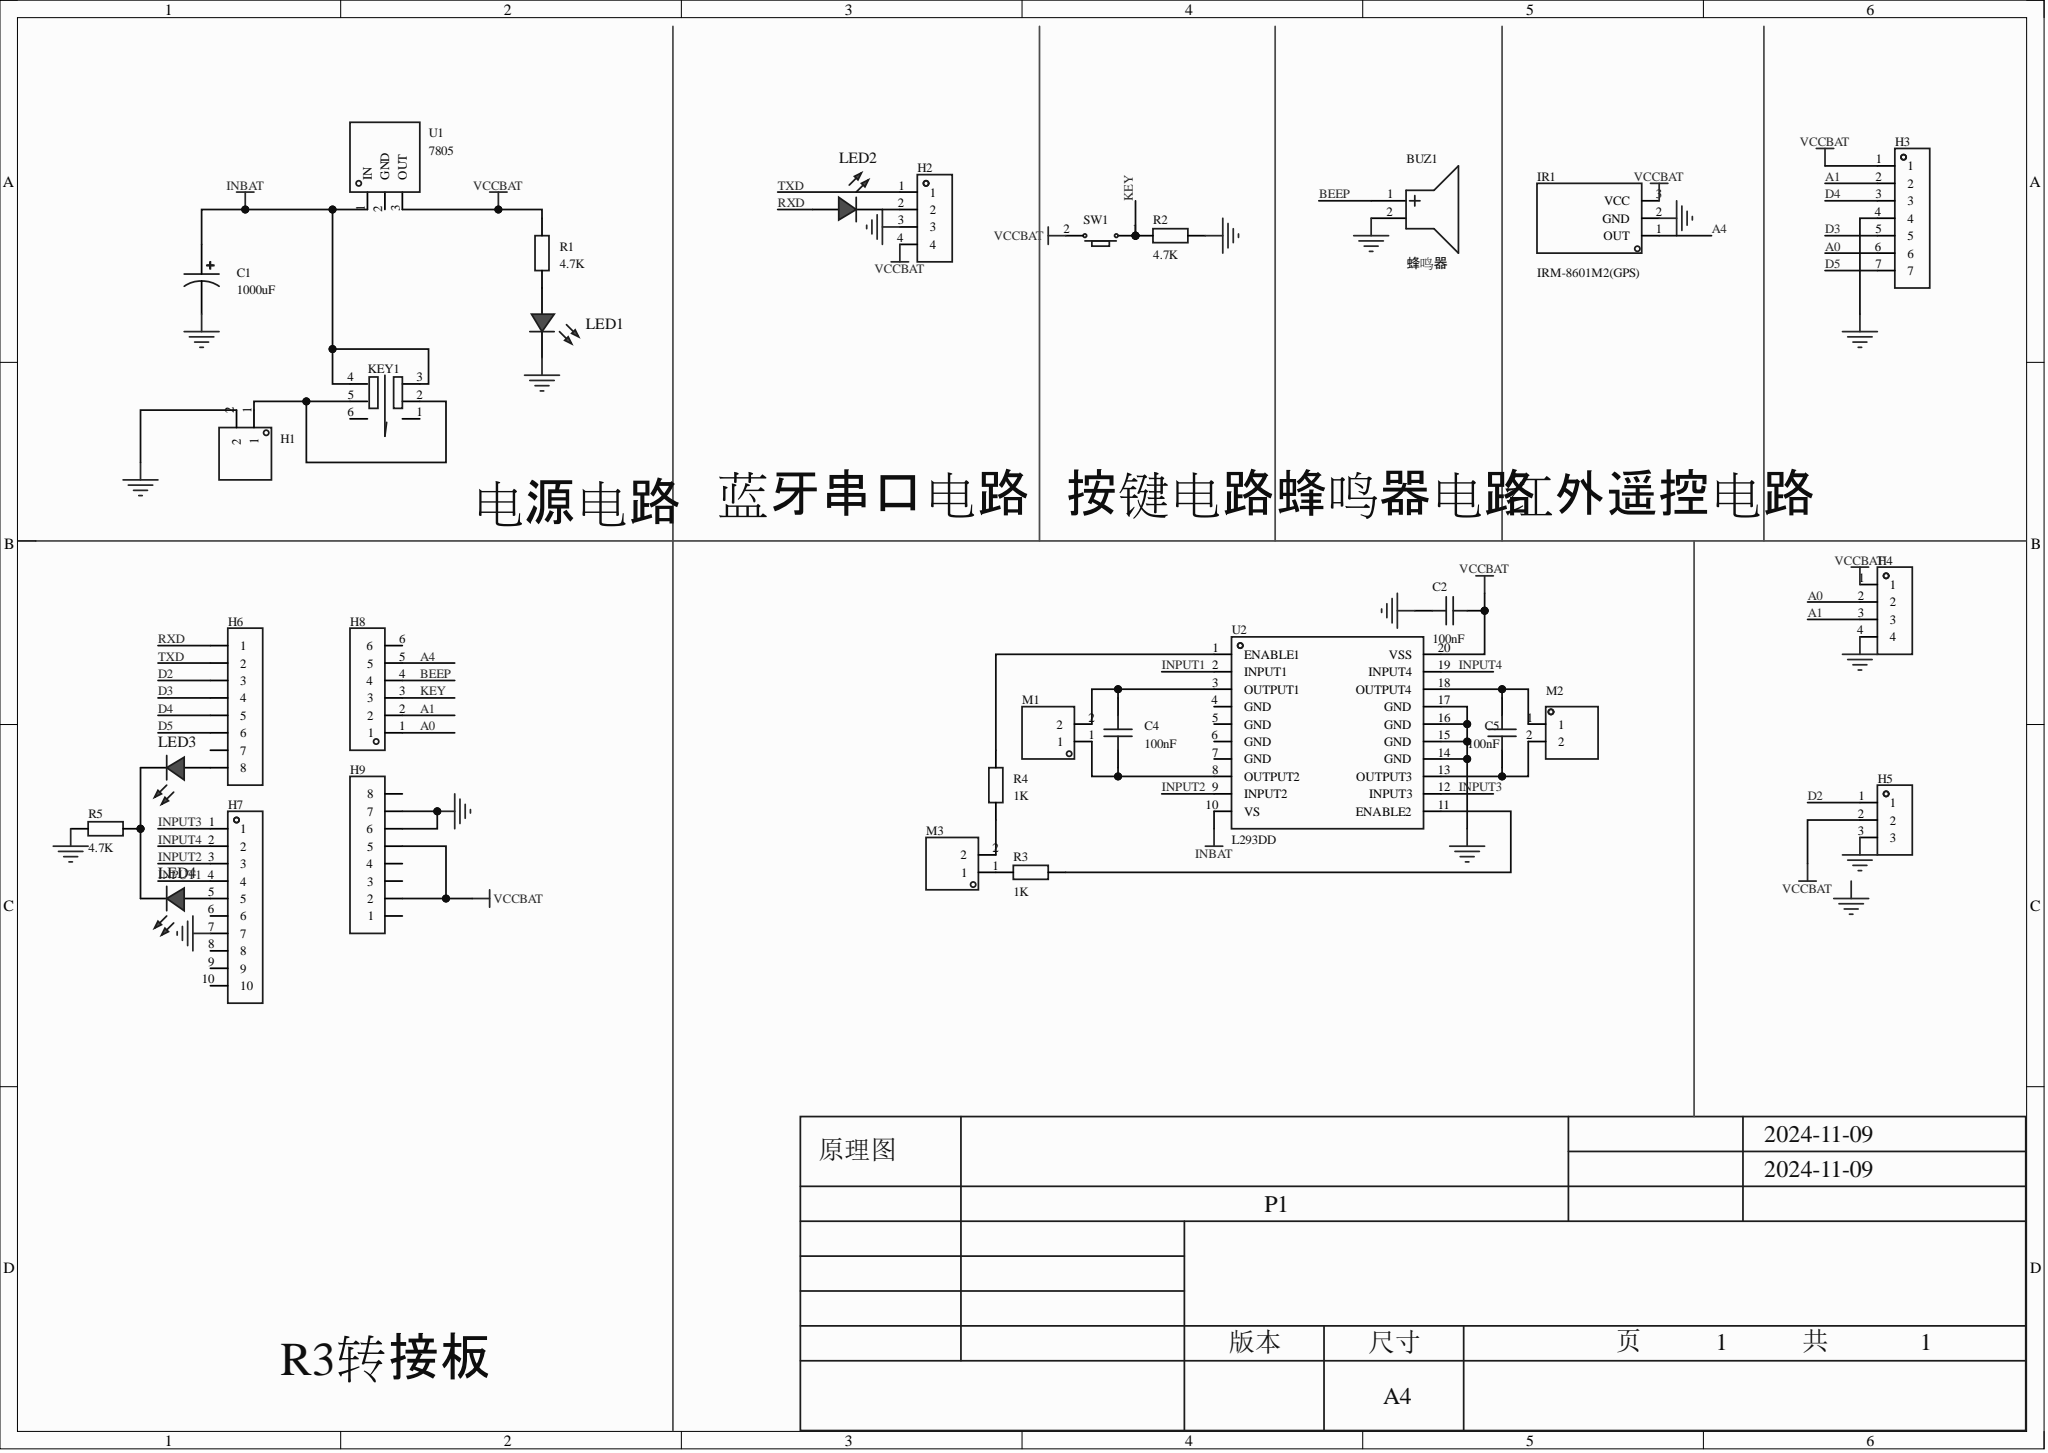Circuit board | Altium Designer | 31 parts | 32 nets
Bill of materials:
Comment,Description,Designator,Footprint,LibRef,Quantity
"蜂鸣器","","BUZ1","BUZ-TH_BD9.0-P5.00-D0.6-FD","蜂鸣器","1"
"1000uF","容值:1000uF;精度:±20%;额定电压:10V;纹波电流:-;等效串联电阻:-;","C1","CAP-TH_BD8.0-P3.50-D0.6-FD","SHW1000UF10V8X12","1"
"100nF","","C2, C4, C5","C0603","CAP_0603","3"
"","","H1, M1, M2, M3","HDR-TH_2P-P2.54-V-M-1","HDR-M_2.54_1x2P","4"
"","","H2, H4","HDR-TH_4P-P2.54-V-F","HDR-F_2.54_1x4P","2"
"","","H3","HDR-TH_7P-P2.54-V-M","HDR-M_2.54_1x7P","1"
"","","H5","HDR-TH_3P-P2.54-V-F","HDR-F_2.54_1x3P","1"
"","","H6, H9","HDR-TH_8P-P2.54-V-F-1","HDR-F_2.54_1x8P","2"
"","","H7","HDR-TH_10P-P2.54-V-F","HDR-F_2.54_1x10P","1"
"","","H8","HDR-TH_6P-P2.54-V-F","HDR-F_2.54_1x6P","1"
"IRM-8601M2(GPS)","","IR1","SENSOR-TH_IRM-8601","IRM-8601M2(GPS)","1"
"自锁开关 5.8Z白灰白260G","耐温260度","KEY1","SW-TH_6P-L5.8-W5.8-P2.00-LS4.5-TR","自锁开关 5.8Z白灰白260G","1"
"","","LED1, LED2, LED3, LED4","LED_0603","LED_0603-R","4"
"4.7K","","R1, R2, R5","R0603","Res_0603","3"
"1K","","R3, R4","R0603","Res_0603","2"
"","","SW1","Key_SMD_3x4x2","Key_SMD_3x4x2","1"
"7805","输出类型:固定;最大输入电压:35V;输出电压:5V;最大输出电流:1.5A;电源纹波抑制比(PSRR):62dB@(120Hz);输出极性:正极;","U1","TO-220-3_L10.2-W4.5-P2.54-L-1","7805","1"
"L293DD","","U2","SOIC-20_L13.0-W7.6-P1.27-LS10.3-BL","L293DD_C2971293","1"
Netlist (Protel format):
[
BUZ1
BUZ-TH_BD9.0-P5.00-D0.6-FD
蜂鸣器



]
[
C1
CAP-TH_BD8.0-P3.50-D0.6-FD
1000uF



]
[
C2
C0603
100nF



]
[
C4
C0603
100nF



]
[
C5
C0603
100nF



]
[
H1
HDR-TH_2P-P2.54-V-M-1




]
[
H2
HDR-TH_4P-P2.54-V-F




]
[
H3
HDR-TH_7P-P2.54-V-M




]
[
H4
HDR-TH_4P-P2.54-V-F




]
[
H5
HDR-TH_3P-P2.54-V-F




]
[
H6
HDR-TH_8P-P2.54-V-F-1




]
[
H7
HDR-TH_10P-P2.54-V-F




]
[
H8
HDR-TH_6P-P2.54-V-F




]
[
H9
HDR-TH_8P-P2.54-V-F-1




]
[
IR1
SENSOR-TH_IRM-8601
IRM-8601M2(GPS)



]
[
KEY1
SW-TH_6P-L5.8-W5.8-P2.00-LS4.5-TR
自锁开关 5.8Z白灰白260G



]
[
LED1
LED_0603




]
[
LED2
LED_0603




]
[
LED3
LED_0603




]
[
LED4
LED_0603




]
[
M1
HDR-TH_2P-P2.54-V-M-1




]
[
M2
HDR-TH_2P-P2.54-V-M-1




]
[
M3
HDR-TH_2P-P2.54-V-M-1




]
[
R1
R0603
4.7K



]
[
R2
R0603
4.7K



]
[
R3
R0603
1K



]
[
R4
R0603
1K



]
[
R5
R0603
4.7K



]
[
SW1
Key_SMD_3x4x2




]
[
U1
TO-220-3_L10.2-W4.5-P2.54-L-1
7805



]
[
U2
SOIC-20_L13.0-W7.6-P1.27-LS10.3-BL
L293DD



]
(
VCCBAT
C2-2
H2-4
H3-1
H4-1
H5-2
H9-2
H9-5
IR1-3
R1-2
SW1-2
U1-3
U2-20
)
(
TXD
H2-1
H6-2
)
(
RXD
H6-1
LED2-2
)
(
NetR4_1
R4-1
U2-1
)
(
NetR3_1
R3-1
U2-11
)
(
NetM3_2
M3-2
R4-2
)
(
NetM3_1
M3-1
R3-2
)
(
NetLED3_1
LED3-1
LED4-1
R5-1
)
(
NetLED1_2
LED1-2
R1-1
)
(
NetH7_5
H7-5
LED4-2
)
(
NetH6_8
H6-8
LED3-2
)
(
NetH2_2
H2-2
LED2-1
)
(
NetH1_1
H1-1
KEY1-2
KEY1-5
)
(
NetC5_2
C5-2
M2-2
U2-13
)
(
NetC5_1
C5-1
M2-1
U2-18
)
(
NetC4_2
C4-2
M1-2
U2-3
)
(
NetC4_1
C4-1
M1-1
U2-8
)
(
KEY
H8-3
R2-2
SW1-1
)
(
INPUT4
H7-2
U2-19
)
(
INPUT3
H7-1
U2-12
)
(
INPUT2
H7-3
U2-9
)
(
INPUT1
H7-4
U2-2
)
(
INBAT
C1-1
KEY1-3
KEY1-4
U1-1
U2-10
)
(
GND
BUZ1-2
C1-2
C2-1
H1-2
H2-3
H3-4
H4-4
H5-3
H7-7
H9-6
H9-7
IR1-2
LED1-1
R2-1
R5-2
U2-14
U2-15
U2-16
U2-17
)
(
D5
H3-7
H6-6
)
(
D4
H3-3
H6-5
)
(
D3
H3-5
H6-4
)
(
D2
H5-1
H6-3
)
(
BEEP
BUZ1-1
H8-4
)
(
A4
H8-5
IR1-1
)
(
A1
H3-2
H4-3
H8-2
)
(
A0
H3-6
H4-2
H8-1
)